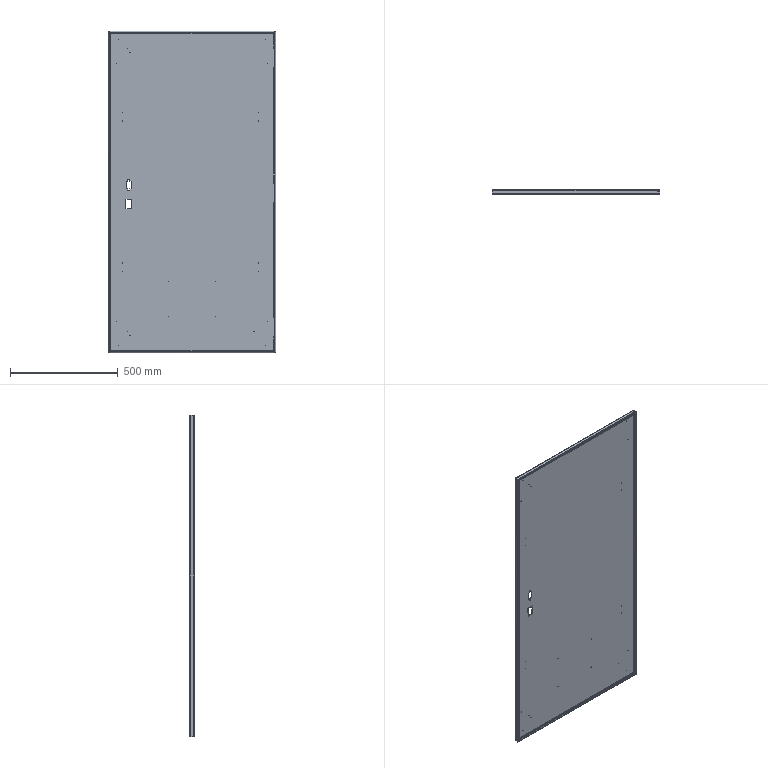Part | NX | features solid 2 | 1 solid | 193 faces | box 777 x 20 x 1495 mm | volume 2527635 mm3 | plane 94 | cylinder 72 | spline 27 | commonest cylinder face diameters 1 x54 4 x8 8 x8 9 x2